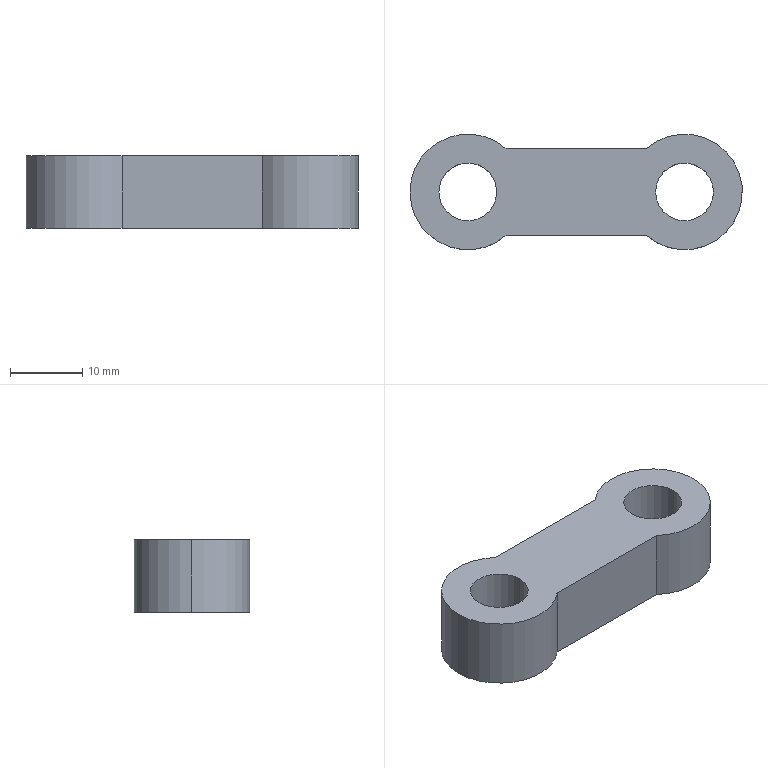Part | SolidWorks | features Extrusion 1 | 1 solid | 11 faces | box 46 x 16 x 10 mm | volume 4895 mm3 | cylinder 7 | plane 4 | commonest cylinder face diameters 8 x4 16 x3
STEP:
#1=CARTESIAN_POINT('',(26.,0.,10.));
#2=VERTEX_POINT('',#1);
#3=CARTESIAN_POINT('',(34.,0.,10.));
#4=VERTEX_POINT('',#3);
#5=CARTESIAN_POINT('',(30.,0.,10.));
#6=DIRECTION('',(0.,0.,1.));
#7=DIRECTION('',(1.,0.,0.));
#8=AXIS2_PLACEMENT_3D('',#5,#6,#7);
#9=CIRCLE('',#8,4.);
#10=EDGE_CURVE('',#2,#4,#9,.T.);
#11=ORIENTED_EDGE('',*,*,#10,.T.);
#12=CARTESIAN_POINT('',(34.,0.,0.));
#13=VERTEX_POINT('',#12);
#14=CARTESIAN_POINT('',(34.,0.,10.));
#15=DIRECTION('',(0.,0.,-1.));
#16=VECTOR('',#15,1000.);
#17=LINE('',#14,#16);
#18=EDGE_CURVE('',#4,#13,#17,.T.);
#19=ORIENTED_EDGE('',*,*,#18,.T.);
#20=CARTESIAN_POINT('',(26.,0.,0.));
#21=VERTEX_POINT('',#20);
#22=CARTESIAN_POINT('',(30.,0.,0.));
#23=DIRECTION('',(0.,0.,1.));
#24=DIRECTION('',(1.,0.,0.));
#25=AXIS2_PLACEMENT_3D('',#22,#23,#24);
#26=CIRCLE('',#25,4.);
#27=EDGE_CURVE('',#21,#13,#26,.T.);
#28=ORIENTED_EDGE('',*,*,#27,.F.);
#29=CARTESIAN_POINT('',(26.,0.,10.));
#30=DIRECTION('',(0.,0.,-1.));
#31=VECTOR('',#30,1000.);
#32=LINE('',#29,#31);
#33=EDGE_CURVE('',#2,#21,#32,.T.);
#34=ORIENTED_EDGE('',*,*,#33,.F.);
#35=EDGE_LOOP('',(#11,#19,#28,#34));
#36=FACE_OUTER_BOUND('',#35,.T.);
#37=CARTESIAN_POINT('',(30.,0.,10.));
#38=DIRECTION('',(0.,0.,-1.));
#39=DIRECTION('',(-1.,0.,0.));
#40=AXIS2_PLACEMENT_3D('',#37,#38,#39);
#41=CYLINDRICAL_SURFACE('',#40,4.);
#42=ADVANCED_FACE('',(#36),#41,.F.);
#43=CARTESIAN_POINT('',(-4.,0.,10.));
#44=VERTEX_POINT('',#43);
#45=CARTESIAN_POINT('',(4.,0.,10.));
#46=VERTEX_POINT('',#45);
#47=CARTESIAN_POINT('',(0.,0.,10.));
#48=DIRECTION('',(0.,0.,1.));
#49=DIRECTION('',(1.,0.,0.));
#50=AXIS2_PLACEMENT_3D('',#47,#48,#49);
#51=CIRCLE('',#50,4.);
#52=EDGE_CURVE('',#44,#46,#51,.T.);
#53=ORIENTED_EDGE('',*,*,#52,.T.);
#54=CARTESIAN_POINT('',(4.,0.,0.));
#55=VERTEX_POINT('',#54);
#56=CARTESIAN_POINT('',(4.,0.,10.));
#57=DIRECTION('',(0.,0.,-1.));
#58=VECTOR('',#57,1000.);
#59=LINE('',#56,#58);
#60=EDGE_CURVE('',#46,#55,#59,.T.);
#61=ORIENTED_EDGE('',*,*,#60,.T.);
#62=CARTESIAN_POINT('',(-4.,0.,0.));
#63=VERTEX_POINT('',#62);
#64=CARTESIAN_POINT('',(0.,0.,0.));
#65=DIRECTION('',(0.,0.,1.));
#66=DIRECTION('',(1.,0.,0.));
#67=AXIS2_PLACEMENT_3D('',#64,#65,#66);
#68=CIRCLE('',#67,4.);
#69=EDGE_CURVE('',#63,#55,#68,.T.);
#70=ORIENTED_EDGE('',*,*,#69,.F.);
#71=CARTESIAN_POINT('',(-4.,0.,10.));
#72=DIRECTION('',(0.,0.,-1.));
#73=VECTOR('',#72,1000.);
#74=LINE('',#71,#73);
#75=EDGE_CURVE('',#44,#63,#74,.T.);
#76=ORIENTED_EDGE('',*,*,#75,.F.);
#77=EDGE_LOOP('',(#53,#61,#70,#76));
#78=FACE_OUTER_BOUND('',#77,.T.);
#79=CARTESIAN_POINT('',(0.,0.,10.));
#80=DIRECTION('',(0.,0.,-1.));
#81=DIRECTION('',(-1.,0.,0.));
#82=AXIS2_PLACEMENT_3D('',#79,#80,#81);
#83=CYLINDRICAL_SURFACE('',#82,4.);
#84=ADVANCED_FACE('',(#78),#83,.F.);
#85=CARTESIAN_POINT('',(-8.,0.,10.));
#86=VERTEX_POINT('',#85);
#87=CARTESIAN_POINT('',(5.292,-6.,10.));
#88=VERTEX_POINT('',#87);
#89=CARTESIAN_POINT('',(0.,0.,10.));
#90=DIRECTION('',(0.,0.,1.));
#91=DIRECTION('',(1.,0.,0.));
#92=AXIS2_PLACEMENT_3D('',#89,#90,#91);
#93=CIRCLE('',#92,8.);
#94=EDGE_CURVE('',#86,#88,#93,.T.);
#95=ORIENTED_EDGE('',*,*,#94,.F.);
#96=CARTESIAN_POINT('',(-8.,0.,0.));
#97=VERTEX_POINT('',#96);
#98=CARTESIAN_POINT('',(-8.,0.,10.));
#99=DIRECTION('',(0.,0.,-1.));
#100=VECTOR('',#99,1000.);
#101=LINE('',#98,#100);
#102=EDGE_CURVE('',#86,#97,#101,.T.);
#103=ORIENTED_EDGE('',*,*,#102,.T.);
#104=CARTESIAN_POINT('',(5.292,-6.,0.));
#105=VERTEX_POINT('',#104);
#106=CARTESIAN_POINT('',(0.,0.,0.));
#107=DIRECTION('',(0.,0.,1.));
#108=DIRECTION('',(1.,0.,0.));
#109=AXIS2_PLACEMENT_3D('',#106,#107,#108);
#110=CIRCLE('',#109,8.);
#111=EDGE_CURVE('',#97,#105,#110,.T.);
#112=ORIENTED_EDGE('',*,*,#111,.T.);
#113=CARTESIAN_POINT('',(5.292,-6.,10.));
#114=DIRECTION('',(0.,0.,-1.));
#115=VECTOR('',#114,1000.);
#116=LINE('',#113,#115);
#117=EDGE_CURVE('',#88,#105,#116,.T.);
#118=ORIENTED_EDGE('',*,*,#117,.F.);
#119=EDGE_LOOP('',(#95,#103,#112,#118));
#120=FACE_OUTER_BOUND('',#119,.T.);
#121=CARTESIAN_POINT('',(0.,0.,10.));
#122=DIRECTION('',(0.,0.,-1.));
#123=DIRECTION('',(-1.,0.,0.));
#124=AXIS2_PLACEMENT_3D('',#121,#122,#123);
#125=CYLINDRICAL_SURFACE('',#124,8.);
#126=ADVANCED_FACE('',(#120),#125,.T.);
#127=ORIENTED_EDGE('',*,*,#52,.F.);
#128=CARTESIAN_POINT('',(0.,0.,10.));
#129=DIRECTION('',(0.,0.,1.));
#130=DIRECTION('',(1.,0.,0.));
#131=AXIS2_PLACEMENT_3D('',#128,#129,#130);
#132=CIRCLE('',#131,4.);
#133=EDGE_CURVE('',#46,#44,#132,.T.);
#134=ORIENTED_EDGE('',*,*,#133,.F.);
#135=EDGE_LOOP('',(#127,#134));
#136=FACE_BOUND('',#135,.T.);
#137=CARTESIAN_POINT('',(5.292,6.,10.));
#138=VERTEX_POINT('',#137);
#139=CARTESIAN_POINT('',(0.,0.,10.));
#140=DIRECTION('',(0.,0.,1.));
#141=DIRECTION('',(1.,0.,0.));
#142=AXIS2_PLACEMENT_3D('',#139,#140,#141);
#143=CIRCLE('',#142,8.);
#144=EDGE_CURVE('',#138,#86,#143,.T.);
#145=ORIENTED_EDGE('',*,*,#144,.T.);
#146=ORIENTED_EDGE('',*,*,#94,.T.);
#147=CARTESIAN_POINT('',(24.708,-6.,10.));
#148=VERTEX_POINT('',#147);
#149=CARTESIAN_POINT('',(5.292,-6.,10.));
#150=DIRECTION('',(1.,0.,0.));
#151=VECTOR('',#150,1000.);
#152=LINE('',#149,#151);
#153=EDGE_CURVE('',#88,#148,#152,.T.);
#154=ORIENTED_EDGE('',*,*,#153,.T.);
#155=CARTESIAN_POINT('',(24.708,6.,10.));
#156=VERTEX_POINT('',#155);
#157=CARTESIAN_POINT('',(30.,0.,10.));
#158=DIRECTION('',(0.,0.,1.));
#159=DIRECTION('',(1.,0.,0.));
#160=AXIS2_PLACEMENT_3D('',#157,#158,#159);
#161=CIRCLE('',#160,8.);
#162=EDGE_CURVE('',#148,#156,#161,.T.);
#163=ORIENTED_EDGE('',*,*,#162,.T.);
#164=CARTESIAN_POINT('',(5.292,6.,10.));
#165=DIRECTION('',(-1.,0.,0.));
#166=VECTOR('',#165,1000.);
#167=LINE('',#164,#166);
#168=EDGE_CURVE('',#156,#138,#167,.T.);
#169=ORIENTED_EDGE('',*,*,#168,.T.);
#170=EDGE_LOOP('',(#145,#146,#154,#163,#169));
#171=FACE_OUTER_BOUND('',#170,.T.);
#172=ORIENTED_EDGE('',*,*,#10,.F.);
#173=CARTESIAN_POINT('',(30.,0.,10.));
#174=DIRECTION('',(0.,0.,1.));
#175=DIRECTION('',(1.,0.,0.));
#176=AXIS2_PLACEMENT_3D('',#173,#174,#175);
#177=CIRCLE('',#176,4.);
#178=EDGE_CURVE('',#4,#2,#177,.T.);
#179=ORIENTED_EDGE('',*,*,#178,.F.);
#180=EDGE_LOOP('',(#172,#179));
#181=FACE_BOUND('',#180,.T.);
#182=CARTESIAN_POINT('',(0.,0.,10.));
#183=DIRECTION('',(0.,0.,1.));
#184=DIRECTION('',(1.,0.,0.));
#185=AXIS2_PLACEMENT_3D('',#182,#183,#184);
#186=PLANE('',#185);
#187=ADVANCED_FACE('',(#136,#171,#181),#186,.T.);
#188=CARTESIAN_POINT('',(5.292,6.,0.));
#189=VERTEX_POINT('',#188);
#190=CARTESIAN_POINT('',(0.,0.,0.));
#191=DIRECTION('',(0.,0.,1.));
#192=DIRECTION('',(1.,0.,0.));
#193=AXIS2_PLACEMENT_3D('',#190,#191,#192);
#194=CIRCLE('',#193,8.);
#195=EDGE_CURVE('',#189,#97,#194,.T.);
#196=ORIENTED_EDGE('',*,*,#195,.F.);
#197=CARTESIAN_POINT('',(24.708,6.,0.));
#198=VERTEX_POINT('',#197);
#199=CARTESIAN_POINT('',(5.292,6.,0.));
#200=DIRECTION('',(-1.,0.,0.));
#201=VECTOR('',#200,1000.);
#202=LINE('',#199,#201);
#203=EDGE_CURVE('',#198,#189,#202,.T.);
#204=ORIENTED_EDGE('',*,*,#203,.F.);
#205=CARTESIAN_POINT('',(24.708,-6.,0.));
#206=VERTEX_POINT('',#205);
#207=CARTESIAN_POINT('',(30.,0.,0.));
#208=DIRECTION('',(0.,0.,1.));
#209=DIRECTION('',(1.,0.,0.));
#210=AXIS2_PLACEMENT_3D('',#207,#208,#209);
#211=CIRCLE('',#210,8.);
#212=EDGE_CURVE('',#206,#198,#211,.T.);
#213=ORIENTED_EDGE('',*,*,#212,.F.);
#214=CARTESIAN_POINT('',(5.292,-6.,0.));
#215=DIRECTION('',(1.,0.,0.));
#216=VECTOR('',#215,1000.);
#217=LINE('',#214,#216);
#218=EDGE_CURVE('',#105,#206,#217,.T.);
#219=ORIENTED_EDGE('',*,*,#218,.F.);
#220=ORIENTED_EDGE('',*,*,#111,.F.);
#221=EDGE_LOOP('',(#196,#204,#213,#219,#220));
#222=FACE_OUTER_BOUND('',#221,.T.);
#223=ORIENTED_EDGE('',*,*,#69,.T.);
#224=CARTESIAN_POINT('',(0.,0.,0.));
#225=DIRECTION('',(0.,0.,1.));
#226=DIRECTION('',(1.,0.,0.));
#227=AXIS2_PLACEMENT_3D('',#224,#225,#226);
#228=CIRCLE('',#227,4.);
#229=EDGE_CURVE('',#55,#63,#228,.T.);
#230=ORIENTED_EDGE('',*,*,#229,.T.);
#231=EDGE_LOOP('',(#223,#230));
#232=FACE_BOUND('',#231,.T.);
#233=ORIENTED_EDGE('',*,*,#27,.T.);
#234=CARTESIAN_POINT('',(30.,0.,0.));
#235=DIRECTION('',(0.,0.,1.));
#236=DIRECTION('',(1.,0.,0.));
#237=AXIS2_PLACEMENT_3D('',#234,#235,#236);
#238=CIRCLE('',#237,4.);
#239=EDGE_CURVE('',#13,#21,#238,.T.);
#240=ORIENTED_EDGE('',*,*,#239,.T.);
#241=EDGE_LOOP('',(#233,#240));
#242=FACE_BOUND('',#241,.T.);
#243=CARTESIAN_POINT('',(0.,0.,0.));
#244=DIRECTION('',(0.,0.,1.));
#245=DIRECTION('',(1.,0.,0.));
#246=AXIS2_PLACEMENT_3D('',#243,#244,#245);
#247=PLANE('',#246);
#248=ADVANCED_FACE('',(#222,#232,#242),#247,.F.);
#249=ORIENTED_EDGE('',*,*,#102,.F.);
#250=ORIENTED_EDGE('',*,*,#144,.F.);
#251=CARTESIAN_POINT('',(5.292,6.,10.));
#252=DIRECTION('',(0.,0.,-1.));
#253=VECTOR('',#252,1000.);
#254=LINE('',#251,#253);
#255=EDGE_CURVE('',#138,#189,#254,.T.);
#256=ORIENTED_EDGE('',*,*,#255,.T.);
#257=ORIENTED_EDGE('',*,*,#195,.T.);
#258=EDGE_LOOP('',(#249,#250,#256,#257));
#259=FACE_OUTER_BOUND('',#258,.T.);
#260=CARTESIAN_POINT('',(0.,0.,10.));
#261=DIRECTION('',(0.,0.,-1.));
#262=DIRECTION('',(-1.,0.,0.));
#263=AXIS2_PLACEMENT_3D('',#260,#261,#262);
#264=CYLINDRICAL_SURFACE('',#263,8.);
#265=ADVANCED_FACE('',(#259),#264,.T.);
#266=ORIENTED_EDGE('',*,*,#218,.T.);
#267=CARTESIAN_POINT('',(24.708,-6.,10.));
#268=DIRECTION('',(0.,0.,-1.));
#269=VECTOR('',#268,1000.);
#270=LINE('',#267,#269);
#271=EDGE_CURVE('',#148,#206,#270,.T.);
#272=ORIENTED_EDGE('',*,*,#271,.F.);
#273=ORIENTED_EDGE('',*,*,#153,.F.);
#274=ORIENTED_EDGE('',*,*,#117,.T.);
#275=EDGE_LOOP('',(#266,#272,#273,#274));
#276=FACE_OUTER_BOUND('',#275,.T.);
#277=CARTESIAN_POINT('',(5.292,-6.,10.));
#278=DIRECTION('',(0.,1.,0.));
#279=DIRECTION('',(0.,0.,1.));
#280=AXIS2_PLACEMENT_3D('',#277,#278,#279);
#281=PLANE('',#280);
#282=ADVANCED_FACE('',(#276),#281,.F.);
#283=ORIENTED_EDGE('',*,*,#212,.T.);
#284=CARTESIAN_POINT('',(24.708,6.,10.));
#285=DIRECTION('',(0.,0.,-1.));
#286=VECTOR('',#285,1000.);
#287=LINE('',#284,#286);
#288=EDGE_CURVE('',#156,#198,#287,.T.);
#289=ORIENTED_EDGE('',*,*,#288,.F.);
#290=ORIENTED_EDGE('',*,*,#162,.F.);
#291=ORIENTED_EDGE('',*,*,#271,.T.);
#292=EDGE_LOOP('',(#283,#289,#290,#291));
#293=FACE_OUTER_BOUND('',#292,.T.);
#294=CARTESIAN_POINT('',(30.,0.,10.));
#295=DIRECTION('',(0.,0.,-1.));
#296=DIRECTION('',(-1.,0.,0.));
#297=AXIS2_PLACEMENT_3D('',#294,#295,#296);
#298=CYLINDRICAL_SURFACE('',#297,8.);
#299=ADVANCED_FACE('',(#293),#298,.T.);
#300=ORIENTED_EDGE('',*,*,#203,.T.);
#301=ORIENTED_EDGE('',*,*,#255,.F.);
#302=ORIENTED_EDGE('',*,*,#168,.F.);
#303=ORIENTED_EDGE('',*,*,#288,.T.);
#304=EDGE_LOOP('',(#300,#301,#302,#303));
#305=FACE_OUTER_BOUND('',#304,.T.);
#306=CARTESIAN_POINT('',(5.292,6.,10.));
#307=DIRECTION('',(0.,-1.,0.));
#308=DIRECTION('',(0.,0.,-1.));
#309=AXIS2_PLACEMENT_3D('',#306,#307,#308);
#310=PLANE('',#309);
#311=ADVANCED_FACE('',(#305),#310,.F.);
#312=ORIENTED_EDGE('',*,*,#60,.F.);
#313=ORIENTED_EDGE('',*,*,#133,.T.);
#314=ORIENTED_EDGE('',*,*,#75,.T.);
#315=ORIENTED_EDGE('',*,*,#229,.F.);
#316=EDGE_LOOP('',(#312,#313,#314,#315));
#317=FACE_OUTER_BOUND('',#316,.T.);
#318=CARTESIAN_POINT('',(0.,0.,10.));
#319=DIRECTION('',(0.,0.,-1.));
#320=DIRECTION('',(-1.,0.,0.));
#321=AXIS2_PLACEMENT_3D('',#318,#319,#320);
#322=CYLINDRICAL_SURFACE('',#321,4.);
#323=ADVANCED_FACE('',(#317),#322,.F.);
#324=ORIENTED_EDGE('',*,*,#18,.F.);
#325=ORIENTED_EDGE('',*,*,#178,.T.);
#326=ORIENTED_EDGE('',*,*,#33,.T.);
#327=ORIENTED_EDGE('',*,*,#239,.F.);
#328=EDGE_LOOP('',(#324,#325,#326,#327));
#329=FACE_OUTER_BOUND('',#328,.T.);
#330=CARTESIAN_POINT('',(30.,0.,10.));
#331=DIRECTION('',(0.,0.,-1.));
#332=DIRECTION('',(-1.,0.,0.));
#333=AXIS2_PLACEMENT_3D('',#330,#331,#332);
#334=CYLINDRICAL_SURFACE('',#333,4.);
#335=ADVANCED_FACE('',(#329),#334,.F.);
#336=CLOSED_SHELL('',(#42,#84,#126,#187,#248,#265,#282,#299,#311,#323,#335));
#337=MANIFOLD_SOLID_BREP('',#336);
#338=CARTESIAN_POINT('',(0.,0.,0.));
#339=DIRECTION('',(0.,0.,1.));
#340=DIRECTION('',(1.,0.,0.));
#341=AXIS2_PLACEMENT_3D('',#338,#339,#340);
#342=(LENGTH_UNIT()NAMED_UNIT(*)SI_UNIT(.MILLI.,.METRE.));
#343=UNCERTAINTY_MEASURE_WITH_UNIT(LENGTH_MEASURE(0.00001),#342,'','');
#344=(NAMED_UNIT(*)PLANE_ANGLE_UNIT()SI_UNIT($,.RADIAN.));
#345=(NAMED_UNIT(*)SI_UNIT($,.STERADIAN.)SOLID_ANGLE_UNIT());
#346=(GEOMETRIC_REPRESENTATION_CONTEXT(3)GLOBAL_UNCERTAINTY_ASSIGNED_CONTEXT((#343))GLOBAL_UNIT_ASSIGNED_CONTEXT((#342,#344,#345))REPRESENTATION_CONTEXT('',''));
#347=ADVANCED_BREP_SHAPE_REPRESENTATION('',(#337,#341),#346);